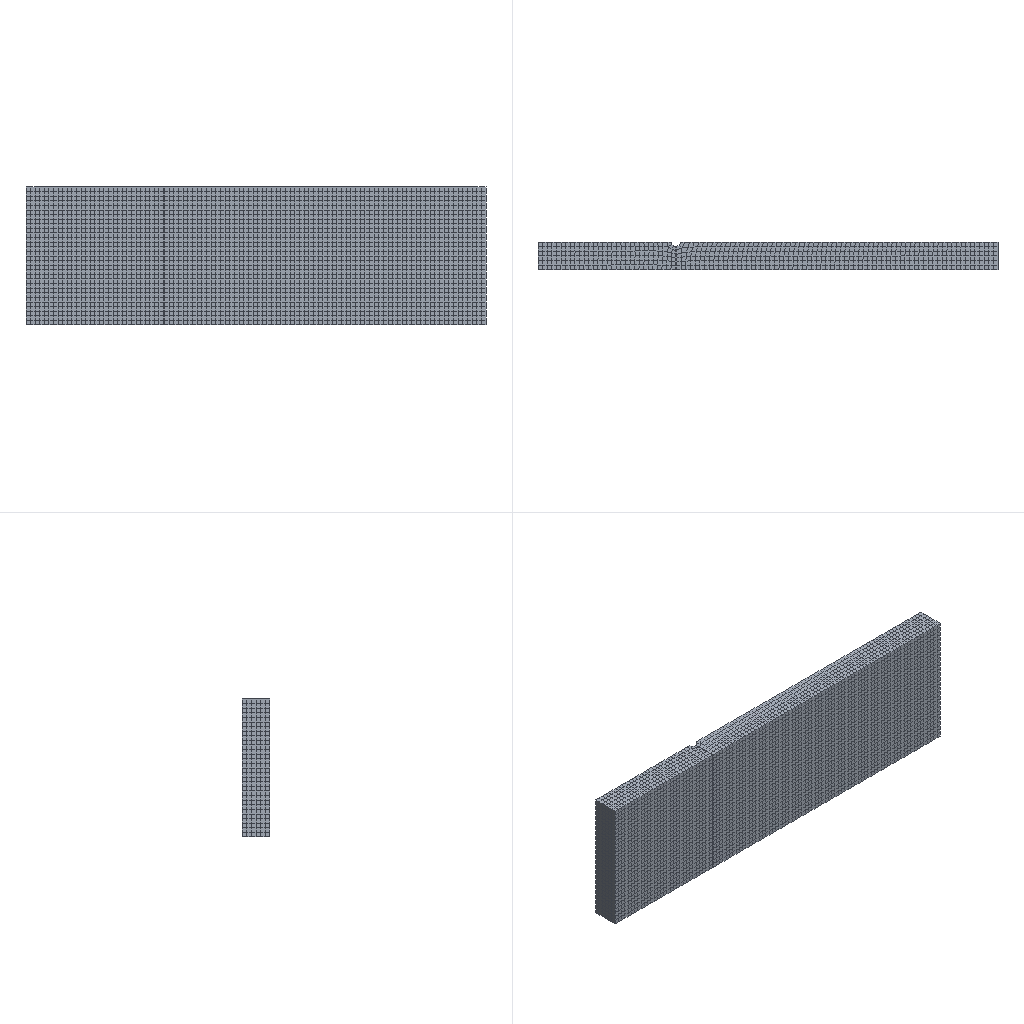Simulation study | abaqus
Set-up summary:
category,name,step,type,value,unit,region
solver,abaqus
solver,version,,,Abaqus/Standard 2020
units,not stated in the deck,,not stated
analysis,deck,,transient,transient
load_step,Step-1,Step-1,transient
load_step,requested,,,1
mesh,nodes,,,23307
mesh,elements,,,19215
element_type,C3D8,,solid,17880
element_type,R3D3,,rigid,6
element_type,R3D4,,rigid,609
element_type,COH3D8,,cohesive,720
load,load commands in deck,,count,1
bc,support commands in deck,,count,7
material,BAN,,in results
material,BAN-CRACK,,in results
check,setup vs results,,match,"per instance, exact: element labels, types and connectivity; labels of the nodes the elements use; coordinates of those nodes at SINGLE_PRECISION in 2 of 2 instance(s)"
Abaqus input file, long lists of numbers shortened:
*Heading
** Job name: Job-1 Model name: Model-1
** Generated by: Abaqus/CAE 2020
*Preprint, echo=NO, model=NO, history=NO, contact=NO
**
** PARTS
**
*Part, name=pmma
*Node
      1,   29.9,           0.,          30.
      2,   29.9,   5.005,          30.
** (22690 more lines like these left out)
*Element, type=C3D8
   1,  1045,  1046,  9262,  8258,    48,    49,   756,   755
   2,  1046,    83,   900,  9262,    49,     1,    50,   756
** (17878 more lines like these left out)
*Element, type=COH3D8
5431,    86,   904, 12398,  3076,     2,    54,  3046,   314
5432,   904,   903, 12399, 12398,    54,    53,  3047,  3046
** (718 more lines like these left out)
*Nset, nset=Set-1, generate
     1,  22692,      1
*Elset, elset=Set-1, generate
     1,  18600,      1
*Nset, nset=Set-64
     1,     2,     3,     4,     5,     6,     7,     8,     9,    10,    11,    12,    13,    14,    15,    16
    17,    18,    19,    20,    21,    22,    23,    24,    25,    26,    27,    28,    29,    30,    31,    32
** (1376 more lines like these left out)
*Elset, elset=Set-64
     1,     2,     3,     4,     5,     6,     7,     8,     9,    10,    11,    12,    13,    14,    15,    16
    17,    18,    19,    20,    21,    22,    23,    24,    25,    26,    27,    28,    29,    30,    31,    32
** (1116 more lines like these left out)
*Nset, nset=Set-65
     1,     2,     6,     7,    11,    12,    13,    14,    50,    51,    52,    53,    54,    55,    56,    57
    58,    59,    60,    61,    62,    63,    64,    65,    66,    67,    68,    69,    70,    71,    72,    73
** (66 more lines like these left out)
*Elset, elset=Set-65, generate
 5431,  6150,     1
** Section: Section-1
*Solid Section, elset=Set-64, material=ban
,
** Section: Section-crack
*Cohesive Section, elset=Set-65, controls=EC-1, material=ban-crack, response=TRACTION SEPARATION
, 1.
*End Part
**
*Part, name=stick
*Node
      1,          -3.,           0.,           0.
      2,          -3.,          30.,           0.
** (612 more lines like these left out)
*Element, type=R3D4
  1,   1,   5,  95,  78
  2,   5,   6,  96,  95
** (607 more lines like these left out)
*Element, type=R3D3
541, 564, 575, 563
542, 585,  72,  71
** (4 more lines like these left out)
*Node
    615,           0.,          30., -1.83697015e-16
*Nset, nset=stick-RefPt_, internal
615,
*Elset, elset=stick, generate
   1,  615,    1
*End Part
**
**
** ASSEMBLY
**
*Assembly, name=Assembly
**
*Instance, name=pmma-1, part=pmma
*End Instance
**
*Instance, name=stick-1, part=stick
         70.,           6.,          15.
*End Instance
**
*Nset, nset=Set-1, instance=pmma-1
    4,    5,    9,   10,   15,   16,   18,   20,  172,  173,  174,  175,  176,  177,  178,  179
  180,  181,  182,  183,  184,  185,  186,  187,  188,  189,  190,  191,  192,  193,  194,  195
** (26 more lines like these left out)
*Elset, elset=Set-1, instance=pmma-1
   223,   251,   279,   307,   335,   363,   391,   419,   447,   475,   503,   531,   559,   587,   615,   616
   617,   618,   619,   620,   756,   757,   758,   759,   760,   896,   897,   898,   899,   900,  1036,  1037
** (21 more lines like these left out)
*Nset, nset=Set-2, instance=stick-1
 615,
*Nset, nset=Set-4, instance=stick-1
 615,
*Nset, nset=Set-5, instance=pmma-1
    4,    5,    9,   10,  172,  173,  174,  175,  176,  177,  178,  179,  180,  181,  182,  183
  184,  185,  186,  187,  188,  189,  190,  191,  192,  193,  194,  195,  196,  197,  198,  199
** (12 more lines like these left out)
*Elset, elset=Set-5, instance=pmma-1
  223,  251,  279,  307,  335,  363,  391,  419,  447,  475,  503,  531,  559,  587,  615,  616
  617,  618,  619,  620,  756,  757,  758,  759,  760,  896,  897,  898,  899,  900, 1036, 1037
** (10 more lines like these left out)
*Nset, nset=Set-6, instance=stick-1
 615,
*Nset, nset=Set-7, instance=pmma-1
    4,    5,    9,   10,  172,  173,  174,  175,  176,  177,  178,  179,  180,  181,  182,  183
  184,  185,  186,  187,  188,  189,  190,  191,  192,  193,  194,  195,  196,  197,  198,  199
** (12 more lines like these left out)
*Elset, elset=Set-7, instance=pmma-1
  223,  251,  279,  307,  335,  363,  391,  419,  447,  475,  503,  531,  559,  587,  615,  616
  617,  618,  619,  620,  756,  757,  758,  759,  760,  896,  897,  898,  899,  900, 1036, 1037
** (10 more lines like these left out)
*Elset, elset=_m_Surf-1_SPOS, internal, instance=stick-1, generate
   1,  577,    1
*Surface, type=ELEMENT, name=m_Surf-1
_m_Surf-1_SPOS, SPOS
*Elset, elset=_s_Surf-1_S4, internal, instance=pmma-1
 11341, 11342, 11343, 11344, 11345, 11346, 11347, 11348, 11349, 11350, 11351, 11352, 11353, 11354, 11355, 11356
 11357, 11358, 11359, 11360, 11361, 11362, 11363, 11364, 11365, 11366, 11367, 11368, 11369, 11370, 11371, 11372
** (63 more lines like these left out)
*Elset, elset=_s_Surf-1_S3, internal, instance=pmma-1
 12361, 12362, 12363, 12364, 12365, 12366, 12367, 12368, 12369, 12370, 12371, 12372, 12373, 12374, 12375, 17581
 17582, 17583, 17584, 17585, 17586, 17587, 17588, 17589, 17590, 17591, 17592, 17593, 17594, 17595, 17596, 17597
** (63 more lines like these left out)
*Surface, type=ELEMENT, name=s_Surf-1
_s_Surf-1_S4, S4
_s_Surf-1_S3, S3
*Rigid Body, ref node=stick-1.stick-RefPt_, elset=stick-1.stick
*Elset, elset=__Int-2_gcs0_5_S3, internal, instance=pmma-1
  6151,  6152,  6153,  6154,  6155,  6156,  6157,  6158,  6159,  6160,  6161,  6162,  6163,  6164,  6165, 12451
 12452, 12453, 12454, 12455, 12456, 12457, 12458, 12459, 12460, 12461, 12462, 12463, 12464, 12465, 17566, 17567
** (1 more lines like these left out)
*Elset, elset=__Int-2_gcs0_5_S4, internal, instance=pmma-1, generate
 12361,  12375,      1
*Surface, type=ELEMENT, name=_Int-2_gcs0_5, internal
__Int-2_gcs0_5_S3, S3
__Int-2_gcs0_5_S4, S4
*Elset, elset=__Int-2_gcs0_6_S4, internal, instance=pmma-1
  151,  152,  153,  154,  155,  156,  157,  158,  159,  160,  161,  162,  163,  164,  165,  166
  167,  168,  169,  170,  171,  172,  173,  174,  175,  176,  177,  178,  179,  180, 2716, 2717
** (2 more lines like these left out)
*Elset, elset=__Int-2_gcs0_6_S3, internal, instance=pmma-1, generate
 181,  195,    1
*Elset, elset=__Int-2_gcs0_6_S2, internal, instance=pmma-1, generate
 2896,  2910,     1
*Surface, type=ELEMENT, name=_Int-2_gcs0_6, internal
__Int-2_gcs0_6_S4, S4
__Int-2_gcs0_6_S3, S3
__Int-2_gcs0_6_S2, S2
*Elset, elset=__Int-2_gcs0_15_S6, internal, instance=pmma-1, generate
 5431,  6145,     6
*Surface, type=ELEMENT, name=_Int-2_gcs0_15, internal
__Int-2_gcs0_15_S6, S6
*Elset, elset=__Int-2_gcs0_20_SPOS, internal, instance=stick-1, generate
   1,  270,    1
*Surface, type=ELEMENT, name=_Int-2_gcs0_20, internal
__Int-2_gcs0_20_SPOS, SPOS
*Elset, elset=__Int-2_gcs0_21_SPOS, internal, instance=stick-1, generate
 271,  540,    1
*Surface, type=ELEMENT, name=_Int-2_gcs0_21, internal
__Int-2_gcs0_21_SPOS, SPOS
*Elset, elset=__Int-2_gcs0_24_SNEG, internal, instance=stick-1, generate
   1,  270,    1
*Surface, type=ELEMENT, name=_Int-2_gcs0_24, internal
__Int-2_gcs0_24_SNEG, SNEG
*Elset, elset=__Int-2_gcs0_25_SNEG, internal, instance=stick-1, generate
 271,  540,    1
*Surface, type=ELEMENT, name=_Int-2_gcs0_25, internal
__Int-2_gcs0_25_SNEG, SNEG
*End Assembly
**
** ELEMENT CONTROLS
**
*Section Controls, name=EC-1, ELEMENT DELETION=YES
1., 1., 1.
*Amplitude, name=Amp-1
             0.,              0.,              1.,              1.
**
** MATERIALS
**
*Material, name=ban
*Density
 1.1e-09,
*Elastic
3160., 0.32
*Material, name=ban-crack
*Damage Initiation, criterion=QUADS
5.,1.,1.
*Damage Evolution, type=DISPLACEMENT
 1e-05,
*Damage Stabilization
0.0001
*Density
 1.1e-09,
*Elastic, type=TRACTION
35000.,25000.,25000.
**
** INTERACTION PROPERTIES
**
*Surface Interaction, name=IntProp-1
1.,
*Friction, slip tolerance=0.005
 0.3,
*Surface Behavior, pressure-overclosure=HARD
*Surface Interaction, name=IntProp-2
1.,
*Cohesive Behavior
**
** INTERACTIONS
**
** Interaction: Int-2
*Contact
*Contact Inclusions, ALL EXTERIOR
*Contact Property Assignment
 ,  , IntProp-1
*Surface Property Assignment, property=GEOMETRIC CORRECTION
_Int-2_gcs0_5, Circumferential, 30., 6., 0.,  30., 6., -1.
_Int-2_gcs0_6, Circumferential, 30., 6., 0.,  30., 6., -1.
_Int-2_gcs0_15, Circumferential, 30., 6., 0.,  30., 6., -1.
_Int-2_gcs0_20, Circumferential, 70., 6., 15.,  70., 5., 15.
_Int-2_gcs0_21, Circumferential, 70., 6., 15.,  70., 5., 15.
_Int-2_gcs0_24, Circumferential, 70., 6., 15.,  70., 5., 15.
_Int-2_gcs0_25, Circumferential, 70., 6., 15.,  70., 5., 15.
** Interaction: Int-3
*Contact Pair, interaction=IntProp-1, type=SURFACE TO SURFACE
s_Surf-1, m_Surf-1
** ----------------------------------------------------------------
**
** STEP: Step-1
**
*Step, name=Step-1, nlgeom=YES, inc=1000
*Dynamic
0.001,1.,1e-05
**
** BOUNDARY CONDITIONS
**
** Name: BC-1 Type: 对称/反对称/完全固定
*Boundary
Set-7, ENCASTRE
** Name: BC-2 Type: 位移/转角
*Boundary, amplitude=Amp-1
Set-6, 1, 1
Set-6, 2, 2, -6.
Set-6, 3, 3
Set-6, 4, 4
Set-6, 5, 5
Set-6, 6, 6
**
** OUTPUT REQUESTS
**
*Restart, write, number interval=1, time marks=NO
**
** FIELD OUTPUT: F-Output-1
**
*Output, field, frequency=1
*Node Output
PHILSM, PSILSM, RF, U, V
*Element Output, directions=YES
E, LE, MISES, PE, PEEQ, S, SDEG, STATUS
*Contact Output
CSDMG, CSTRESS
**
** HISTORY OUTPUT: H-Output-1
**
*Output, history, variable=PRESELECT, number interval=200, time marks=NO
*End Step
Results summary:
result,step,,partial,increments=21 time=0.2047/1.0
result,analysis,,,transient
result,last_loadstep,,,1
result,primary field,,,U
result,reaction total,,FX,0.0,model units
result,reaction total,,FY,-0.0,model units
result,reaction total,,FZ,-0.0,model units